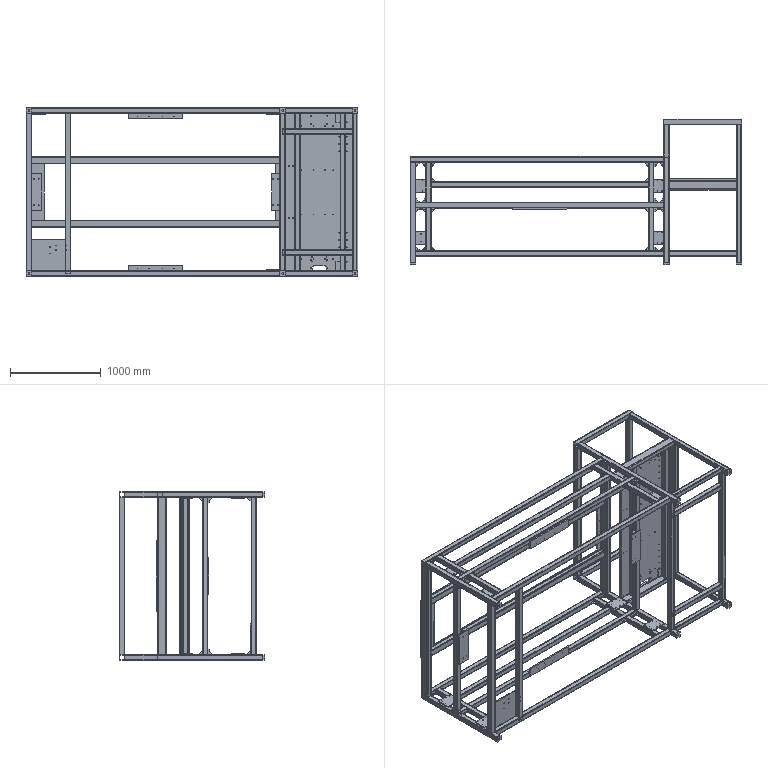Part | SolidWorks | features Gusset 74, WeldCornerFeat 36, HoleWzd 26, WeldMemberFeat 17, ICE 13, MirrorPattern 10, LPattern 7, Fillet 1, WeldmentFeature 1 | 124 solids | 2216 faces | box 3660 x 1605 x 1860 mm | volume 102042670 mm3 | cylinder 1114 | plane 1059 | cone 43 | commonest cylinder face diameters 5 x368 6.4 x140 12.8 x140 6.8 x120 8.5 x84 20 x81